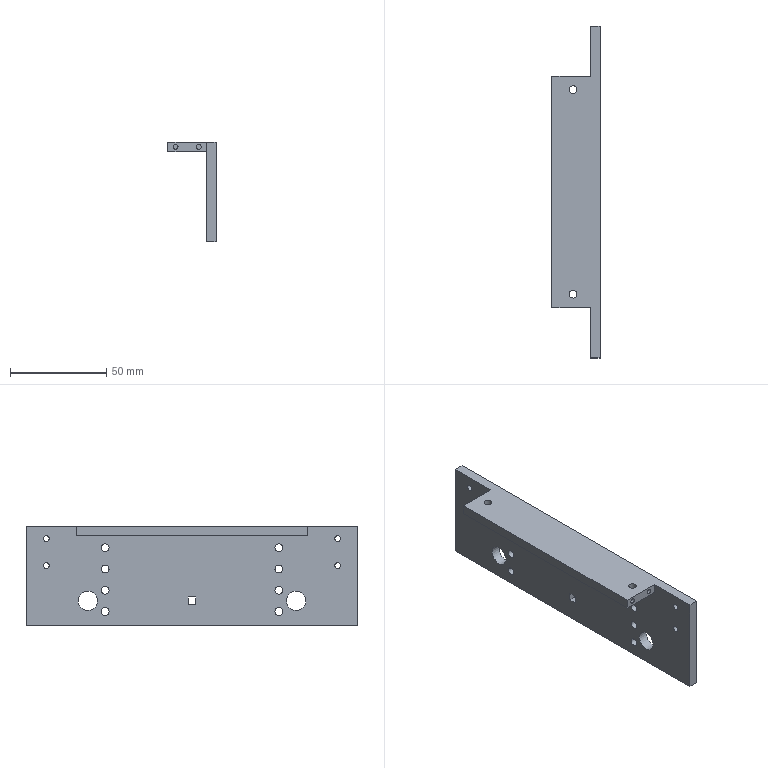Part | STEP file | 1-40.11 | 1 solid | 38 faces | box 25 x 172 x 51.75 mm | volume 54650 mm3 | cylinder 20 | plane 18 | commonest cylinder face diameters 4 x10 3 x4 2.5 x2 2.54 x2 10 x2